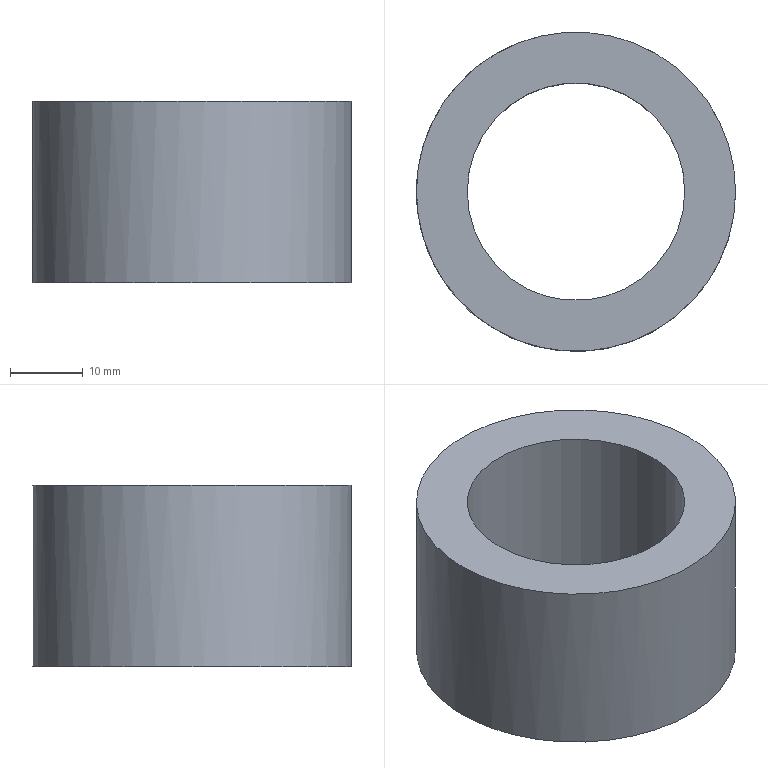Part | NX | features CYLINDER 1, DATUM_CSYS 1, HOLE PACKAGE 1, SIMPLE HOLE 1 | 1 solid | 4 faces | box 44.01 x 44.01 x 24.99 mm | volume 20351 mm3 | plane 2 | cylinder 2 | commonest cylinder face diameters 30 x1 44.01 x1
STEP:
#1=CARTESIAN_POINT('',(15.,0.,24.99));
#2=VERTEX_POINT('',#1);
#3=CARTESIAN_POINT('',(0.,0.,24.99));
#4=DIRECTION('',(0.,0.,1.));
#5=DIRECTION('',(1.,0.,0.));
#6=AXIS2_PLACEMENT_3D('',#3,#4,#5);
#7=CIRCLE('',#6,15.);
#8=EDGE_CURVE('',#2,#2,#7,.T.);
#9=ORIENTED_EDGE('',*,*,#8,.F.);
#10=EDGE_LOOP('',(#9));
#11=FACE_BOUND('',#10,.T.);
#12=CARTESIAN_POINT('',(-22.005,0.,24.99));
#13=VERTEX_POINT('',#12);
#14=CARTESIAN_POINT('',(0.,0.,24.99));
#15=DIRECTION('',(0.,0.,-1.));
#16=DIRECTION('',(-1.,0.,0.));
#17=AXIS2_PLACEMENT_3D('',#14,#15,#16);
#18=CIRCLE('',#17,22.005);
#19=EDGE_CURVE('',#13,#13,#18,.T.);
#20=ORIENTED_EDGE('',*,*,#19,.F.);
#21=EDGE_LOOP('',(#20));
#22=FACE_BOUND('',#21,.T.);
#23=CARTESIAN_POINT('',(0.,0.,24.99));
#24=DIRECTION('',(0.,0.,1.));
#25=DIRECTION('',(1.,0.,0.));
#26=AXIS2_PLACEMENT_3D('',#23,#24,#25);
#27=PLANE('',#26);
#28=ADVANCED_FACE('',(#11,#22),#27,.T.);
#29=CARTESIAN_POINT('',(15.,0.,0.));
#30=VERTEX_POINT('',#29);
#31=CARTESIAN_POINT('',(0.,0.,0.));
#32=DIRECTION('',(0.,0.,1.));
#33=DIRECTION('',(1.,0.,0.));
#34=AXIS2_PLACEMENT_3D('',#31,#32,#33);
#35=CIRCLE('',#34,15.);
#36=EDGE_CURVE('',#30,#30,#35,.T.);
#37=ORIENTED_EDGE('',*,*,#36,.T.);
#38=EDGE_LOOP('',(#37));
#39=FACE_BOUND('',#38,.T.);
#40=CARTESIAN_POINT('',(22.005,0.,0.));
#41=VERTEX_POINT('',#40);
#42=CARTESIAN_POINT('',(0.,0.,0.));
#43=DIRECTION('',(0.,0.,1.));
#44=DIRECTION('',(1.,0.,0.));
#45=AXIS2_PLACEMENT_3D('',#42,#43,#44);
#46=CIRCLE('',#45,22.005);
#47=EDGE_CURVE('',#41,#41,#46,.T.);
#48=ORIENTED_EDGE('',*,*,#47,.F.);
#49=EDGE_LOOP('',(#48));
#50=FACE_BOUND('',#49,.T.);
#51=CARTESIAN_POINT('',(0.,0.,0.));
#52=DIRECTION('',(0.,0.,-1.));
#53=DIRECTION('',(-1.,0.,0.));
#54=AXIS2_PLACEMENT_3D('',#51,#52,#53);
#55=PLANE('',#54);
#56=ADVANCED_FACE('',(#39,#50),#55,.T.);
#57=ORIENTED_EDGE('',*,*,#19,.T.);
#58=EDGE_LOOP('',(#57));
#59=FACE_BOUND('',#58,.T.);
#60=ORIENTED_EDGE('',*,*,#47,.T.);
#61=EDGE_LOOP('',(#60));
#62=FACE_BOUND('',#61,.T.);
#63=CARTESIAN_POINT('',(0.,0.,0.));
#64=DIRECTION('',(0.,0.,1.));
#65=DIRECTION('',(1.,0.,0.));
#66=AXIS2_PLACEMENT_3D('',#63,#64,#65);
#67=CYLINDRICAL_SURFACE('',#66,22.005);
#68=ADVANCED_FACE('',(#59,#62),#67,.T.);
#69=ORIENTED_EDGE('',*,*,#8,.T.);
#70=EDGE_LOOP('',(#69));
#71=FACE_BOUND('',#70,.T.);
#72=ORIENTED_EDGE('',*,*,#36,.F.);
#73=EDGE_LOOP('',(#72));
#74=FACE_BOUND('',#73,.T.);
#75=CARTESIAN_POINT('',(0.,0.,0.));
#76=DIRECTION('',(0.,0.,1.));
#77=DIRECTION('',(1.,0.,0.));
#78=AXIS2_PLACEMENT_3D('',#75,#76,#77);
#79=CYLINDRICAL_SURFACE('',#78,15.);
#80=ADVANCED_FACE('',(#71,#74),#79,.F.);
#81=CLOSED_SHELL('',(#28,#56,#68,#80));
#82=MANIFOLD_SOLID_BREP('',#81);
#83=(LENGTH_UNIT()NAMED_UNIT(*)SI_UNIT(.MILLI.,.METRE.));
#84=UNCERTAINTY_MEASURE_WITH_UNIT(LENGTH_MEASURE(0.00001),#83,'','');
#85=(NAMED_UNIT(*)PLANE_ANGLE_UNIT()SI_UNIT($,.RADIAN.));
#86=(NAMED_UNIT(*)SI_UNIT($,.STERADIAN.)SOLID_ANGLE_UNIT());
#87=(GEOMETRIC_REPRESENTATION_CONTEXT(3)GLOBAL_UNCERTAINTY_ASSIGNED_CONTEXT((#84))GLOBAL_UNIT_ASSIGNED_CONTEXT((#83,#85,#86))REPRESENTATION_CONTEXT('',''));
#88=ADVANCED_BREP_SHAPE_REPRESENTATION('',(#82),#87);